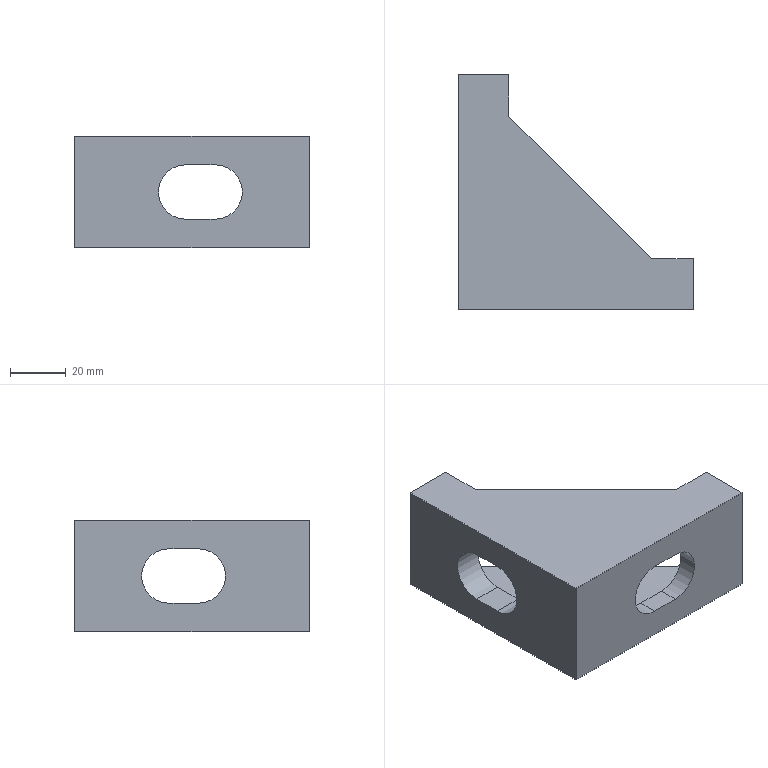Part | STEP file | jiaoma | 1 solid | 24 faces | box 84 x 84 x 40 mm | volume 78299 mm3 | plane 20 | cylinder 4 | commonest cylinder face diameters 19.5 x4